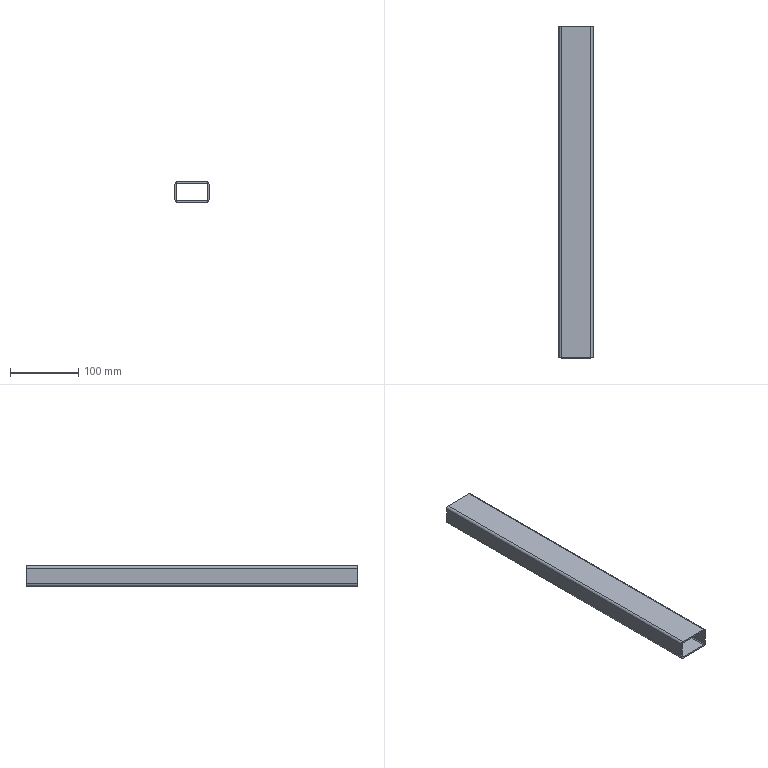Part | SolidWorks | features Extrusion 1 | 1 solid | 18 faces | box 50 x 488 x 30 mm | volume 164826 mm3 | plane 10 | cylinder 8 | commonest cylinder face diameters 2.3 x4 6.9 x4
STEP:
#1=CARTESIAN_POINT('',(25.,488.,-11.55));
#2=VERTEX_POINT('',#1);
#3=CARTESIAN_POINT('',(21.55,488.,-15.));
#4=VERTEX_POINT('',#3);
#5=CARTESIAN_POINT('',(21.55,488.,-11.55));
#6=DIRECTION('',(0.,1.,0.));
#7=DIRECTION('',(0.,0.,-1.));
#8=AXIS2_PLACEMENT_3D('',#5,#6,#7);
#9=CIRCLE('',#8,3.45);
#10=EDGE_CURVE('',#2,#4,#9,.T.);
#11=ORIENTED_EDGE('',*,*,#10,.T.);
#12=CARTESIAN_POINT('',(-21.55,488.,-15.));
#13=VERTEX_POINT('',#12);
#14=CARTESIAN_POINT('',(-21.55,488.,-15.));
#15=DIRECTION('',(-1.,0.,0.));
#16=VECTOR('',#15,1000.);
#17=LINE('',#14,#16);
#18=EDGE_CURVE('',#4,#13,#17,.T.);
#19=ORIENTED_EDGE('',*,*,#18,.T.);
#20=CARTESIAN_POINT('',(-25.,488.,-11.55));
#21=VERTEX_POINT('',#20);
#22=CARTESIAN_POINT('',(-21.55,488.,-11.55));
#23=DIRECTION('',(0.,1.,0.));
#24=DIRECTION('',(0.,0.,-1.));
#25=AXIS2_PLACEMENT_3D('',#22,#23,#24);
#26=CIRCLE('',#25,3.45);
#27=EDGE_CURVE('',#13,#21,#26,.T.);
#28=ORIENTED_EDGE('',*,*,#27,.T.);
#29=CARTESIAN_POINT('',(-25.,488.,11.55));
#30=VERTEX_POINT('',#29);
#31=CARTESIAN_POINT('',(-25.,488.,11.55));
#32=DIRECTION('',(0.,0.,1.));
#33=VECTOR('',#32,1000.);
#34=LINE('',#31,#33);
#35=EDGE_CURVE('',#21,#30,#34,.T.);
#36=ORIENTED_EDGE('',*,*,#35,.T.);
#37=CARTESIAN_POINT('',(-21.55,488.,15.));
#38=VERTEX_POINT('',#37);
#39=CARTESIAN_POINT('',(-21.55,488.,11.55));
#40=DIRECTION('',(0.,1.,0.));
#41=DIRECTION('',(0.,0.,-1.));
#42=AXIS2_PLACEMENT_3D('',#39,#40,#41);
#43=CIRCLE('',#42,3.45);
#44=EDGE_CURVE('',#30,#38,#43,.T.);
#45=ORIENTED_EDGE('',*,*,#44,.T.);
#46=CARTESIAN_POINT('',(21.55,488.,15.));
#47=VERTEX_POINT('',#46);
#48=CARTESIAN_POINT('',(-21.55,488.,15.));
#49=DIRECTION('',(1.,0.,0.));
#50=VECTOR('',#49,1000.);
#51=LINE('',#48,#50);
#52=EDGE_CURVE('',#38,#47,#51,.T.);
#53=ORIENTED_EDGE('',*,*,#52,.T.);
#54=CARTESIAN_POINT('',(25.,488.,11.55));
#55=VERTEX_POINT('',#54);
#56=CARTESIAN_POINT('',(21.55,488.,11.55));
#57=DIRECTION('',(0.,1.,0.));
#58=DIRECTION('',(0.,0.,1.));
#59=AXIS2_PLACEMENT_3D('',#56,#57,#58);
#60=CIRCLE('',#59,3.45);
#61=EDGE_CURVE('',#47,#55,#60,.T.);
#62=ORIENTED_EDGE('',*,*,#61,.T.);
#63=CARTESIAN_POINT('',(25.,488.,11.55));
#64=DIRECTION('',(0.,0.,-1.));
#65=VECTOR('',#64,1000.);
#66=LINE('',#63,#65);
#67=EDGE_CURVE('',#55,#2,#66,.T.);
#68=ORIENTED_EDGE('',*,*,#67,.T.);
#69=EDGE_LOOP('',(#11,#19,#28,#36,#45,#53,#62,#68));
#70=FACE_OUTER_BOUND('',#69,.T.);
#71=CARTESIAN_POINT('',(-22.7,488.,11.55));
#72=VERTEX_POINT('',#71);
#73=CARTESIAN_POINT('',(-21.55,488.,12.7));
#74=VERTEX_POINT('',#73);
#75=CARTESIAN_POINT('',(-21.55,488.,11.55));
#76=DIRECTION('',(0.,1.,0.));
#77=DIRECTION('',(0.,0.,-1.));
#78=AXIS2_PLACEMENT_3D('',#75,#76,#77);
#79=CIRCLE('',#78,1.15);
#80=EDGE_CURVE('',#72,#74,#79,.T.);
#81=ORIENTED_EDGE('',*,*,#80,.F.);
#82=CARTESIAN_POINT('',(-22.7,488.,-11.55));
#83=VERTEX_POINT('',#82);
#84=CARTESIAN_POINT('',(-22.7,488.,11.55));
#85=DIRECTION('',(0.,0.,1.));
#86=VECTOR('',#85,1000.);
#87=LINE('',#84,#86);
#88=EDGE_CURVE('',#83,#72,#87,.T.);
#89=ORIENTED_EDGE('',*,*,#88,.F.);
#90=CARTESIAN_POINT('',(-21.55,488.,-12.7));
#91=VERTEX_POINT('',#90);
#92=CARTESIAN_POINT('',(-21.55,488.,-11.55));
#93=DIRECTION('',(0.,1.,0.));
#94=DIRECTION('',(0.,0.,-1.));
#95=AXIS2_PLACEMENT_3D('',#92,#93,#94);
#96=CIRCLE('',#95,1.15);
#97=EDGE_CURVE('',#91,#83,#96,.T.);
#98=ORIENTED_EDGE('',*,*,#97,.F.);
#99=CARTESIAN_POINT('',(21.55,488.,-12.7));
#100=VERTEX_POINT('',#99);
#101=CARTESIAN_POINT('',(-21.55,488.,-12.7));
#102=DIRECTION('',(-1.,0.,0.));
#103=VECTOR('',#102,1000.);
#104=LINE('',#101,#103);
#105=EDGE_CURVE('',#100,#91,#104,.T.);
#106=ORIENTED_EDGE('',*,*,#105,.F.);
#107=CARTESIAN_POINT('',(22.7,488.,-11.55));
#108=VERTEX_POINT('',#107);
#109=CARTESIAN_POINT('',(21.55,488.,-11.55));
#110=DIRECTION('',(0.,1.,0.));
#111=DIRECTION('',(0.,0.,-1.));
#112=AXIS2_PLACEMENT_3D('',#109,#110,#111);
#113=CIRCLE('',#112,1.15);
#114=EDGE_CURVE('',#108,#100,#113,.T.);
#115=ORIENTED_EDGE('',*,*,#114,.F.);
#116=CARTESIAN_POINT('',(22.7,488.,11.55));
#117=VERTEX_POINT('',#116);
#118=CARTESIAN_POINT('',(22.7,488.,11.55));
#119=DIRECTION('',(0.,0.,-1.));
#120=VECTOR('',#119,1000.);
#121=LINE('',#118,#120);
#122=EDGE_CURVE('',#117,#108,#121,.T.);
#123=ORIENTED_EDGE('',*,*,#122,.F.);
#124=CARTESIAN_POINT('',(21.55,488.,12.7));
#125=VERTEX_POINT('',#124);
#126=CARTESIAN_POINT('',(21.55,488.,11.55));
#127=DIRECTION('',(0.,1.,0.));
#128=DIRECTION('',(0.,0.,1.));
#129=AXIS2_PLACEMENT_3D('',#126,#127,#128);
#130=CIRCLE('',#129,1.15);
#131=EDGE_CURVE('',#125,#117,#130,.T.);
#132=ORIENTED_EDGE('',*,*,#131,.F.);
#133=CARTESIAN_POINT('',(-21.55,488.,12.7));
#134=DIRECTION('',(1.,0.,0.));
#135=VECTOR('',#134,1000.);
#136=LINE('',#133,#135);
#137=EDGE_CURVE('',#74,#125,#136,.T.);
#138=ORIENTED_EDGE('',*,*,#137,.F.);
#139=EDGE_LOOP('',(#81,#89,#98,#106,#115,#123,#132,#138));
#140=FACE_BOUND('',#139,.T.);
#141=CARTESIAN_POINT('',(21.55,488.,-11.55));
#142=DIRECTION('',(0.,-1.,0.));
#143=DIRECTION('',(0.,0.,-1.));
#144=AXIS2_PLACEMENT_3D('',#141,#142,#143);
#145=PLANE('',#144);
#146=ADVANCED_FACE('',(#70,#140),#145,.F.);
#147=CARTESIAN_POINT('',(25.,0.,-11.55));
#148=VERTEX_POINT('',#147);
#149=CARTESIAN_POINT('',(21.55,0.,-15.));
#150=VERTEX_POINT('',#149);
#151=CARTESIAN_POINT('',(21.55,0.,-11.55));
#152=DIRECTION('',(0.,1.,0.));
#153=DIRECTION('',(0.,0.,-1.));
#154=AXIS2_PLACEMENT_3D('',#151,#152,#153);
#155=CIRCLE('',#154,3.45);
#156=EDGE_CURVE('',#148,#150,#155,.T.);
#157=ORIENTED_EDGE('',*,*,#156,.F.);
#158=CARTESIAN_POINT('',(25.,0.,11.55));
#159=VERTEX_POINT('',#158);
#160=CARTESIAN_POINT('',(25.,0.,11.55));
#161=DIRECTION('',(0.,0.,-1.));
#162=VECTOR('',#161,1000.);
#163=LINE('',#160,#162);
#164=EDGE_CURVE('',#159,#148,#163,.T.);
#165=ORIENTED_EDGE('',*,*,#164,.F.);
#166=CARTESIAN_POINT('',(21.55,0.,15.));
#167=VERTEX_POINT('',#166);
#168=CARTESIAN_POINT('',(21.55,0.,11.55));
#169=DIRECTION('',(0.,1.,0.));
#170=DIRECTION('',(0.,0.,1.));
#171=AXIS2_PLACEMENT_3D('',#168,#169,#170);
#172=CIRCLE('',#171,3.45);
#173=EDGE_CURVE('',#167,#159,#172,.T.);
#174=ORIENTED_EDGE('',*,*,#173,.F.);
#175=CARTESIAN_POINT('',(-21.55,0.,15.));
#176=VERTEX_POINT('',#175);
#177=CARTESIAN_POINT('',(-21.55,0.,15.));
#178=DIRECTION('',(1.,0.,0.));
#179=VECTOR('',#178,1000.);
#180=LINE('',#177,#179);
#181=EDGE_CURVE('',#176,#167,#180,.T.);
#182=ORIENTED_EDGE('',*,*,#181,.F.);
#183=CARTESIAN_POINT('',(-25.,0.,11.55));
#184=VERTEX_POINT('',#183);
#185=CARTESIAN_POINT('',(-21.55,0.,11.55));
#186=DIRECTION('',(0.,1.,0.));
#187=DIRECTION('',(0.,0.,-1.));
#188=AXIS2_PLACEMENT_3D('',#185,#186,#187);
#189=CIRCLE('',#188,3.45);
#190=EDGE_CURVE('',#184,#176,#189,.T.);
#191=ORIENTED_EDGE('',*,*,#190,.F.);
#192=CARTESIAN_POINT('',(-25.,0.,-11.55));
#193=VERTEX_POINT('',#192);
#194=CARTESIAN_POINT('',(-25.,0.,11.55));
#195=DIRECTION('',(0.,0.,1.));
#196=VECTOR('',#195,1000.);
#197=LINE('',#194,#196);
#198=EDGE_CURVE('',#193,#184,#197,.T.);
#199=ORIENTED_EDGE('',*,*,#198,.F.);
#200=CARTESIAN_POINT('',(-21.55,0.,-15.));
#201=VERTEX_POINT('',#200);
#202=CARTESIAN_POINT('',(-21.55,0.,-11.55));
#203=DIRECTION('',(0.,1.,0.));
#204=DIRECTION('',(0.,0.,-1.));
#205=AXIS2_PLACEMENT_3D('',#202,#203,#204);
#206=CIRCLE('',#205,3.45);
#207=EDGE_CURVE('',#201,#193,#206,.T.);
#208=ORIENTED_EDGE('',*,*,#207,.F.);
#209=CARTESIAN_POINT('',(-21.55,0.,-15.));
#210=DIRECTION('',(-1.,0.,0.));
#211=VECTOR('',#210,1000.);
#212=LINE('',#209,#211);
#213=EDGE_CURVE('',#150,#201,#212,.T.);
#214=ORIENTED_EDGE('',*,*,#213,.F.);
#215=EDGE_LOOP('',(#157,#165,#174,#182,#191,#199,#208,#214));
#216=FACE_OUTER_BOUND('',#215,.T.);
#217=CARTESIAN_POINT('',(-22.7,0.,-11.55));
#218=VERTEX_POINT('',#217);
#219=CARTESIAN_POINT('',(-22.7,0.,11.55));
#220=VERTEX_POINT('',#219);
#221=CARTESIAN_POINT('',(-22.7,0.,11.55));
#222=DIRECTION('',(0.,0.,1.));
#223=VECTOR('',#222,1000.);
#224=LINE('',#221,#223);
#225=EDGE_CURVE('',#218,#220,#224,.T.);
#226=ORIENTED_EDGE('',*,*,#225,.T.);
#227=CARTESIAN_POINT('',(-21.55,0.,12.7));
#228=VERTEX_POINT('',#227);
#229=CARTESIAN_POINT('',(-21.55,0.,11.55));
#230=DIRECTION('',(0.,1.,0.));
#231=DIRECTION('',(0.,0.,-1.));
#232=AXIS2_PLACEMENT_3D('',#229,#230,#231);
#233=CIRCLE('',#232,1.15);
#234=EDGE_CURVE('',#220,#228,#233,.T.);
#235=ORIENTED_EDGE('',*,*,#234,.T.);
#236=CARTESIAN_POINT('',(21.55,0.,12.7));
#237=VERTEX_POINT('',#236);
#238=CARTESIAN_POINT('',(-21.55,0.,12.7));
#239=DIRECTION('',(1.,0.,0.));
#240=VECTOR('',#239,1000.);
#241=LINE('',#238,#240);
#242=EDGE_CURVE('',#228,#237,#241,.T.);
#243=ORIENTED_EDGE('',*,*,#242,.T.);
#244=CARTESIAN_POINT('',(22.7,0.,11.55));
#245=VERTEX_POINT('',#244);
#246=CARTESIAN_POINT('',(21.55,0.,11.55));
#247=DIRECTION('',(0.,1.,0.));
#248=DIRECTION('',(0.,0.,1.));
#249=AXIS2_PLACEMENT_3D('',#246,#247,#248);
#250=CIRCLE('',#249,1.15);
#251=EDGE_CURVE('',#237,#245,#250,.T.);
#252=ORIENTED_EDGE('',*,*,#251,.T.);
#253=CARTESIAN_POINT('',(22.7,0.,-11.55));
#254=VERTEX_POINT('',#253);
#255=CARTESIAN_POINT('',(22.7,0.,11.55));
#256=DIRECTION('',(0.,0.,-1.));
#257=VECTOR('',#256,1000.);
#258=LINE('',#255,#257);
#259=EDGE_CURVE('',#245,#254,#258,.T.);
#260=ORIENTED_EDGE('',*,*,#259,.T.);
#261=CARTESIAN_POINT('',(21.55,0.,-12.7));
#262=VERTEX_POINT('',#261);
#263=CARTESIAN_POINT('',(21.55,0.,-11.55));
#264=DIRECTION('',(0.,1.,0.));
#265=DIRECTION('',(0.,0.,-1.));
#266=AXIS2_PLACEMENT_3D('',#263,#264,#265);
#267=CIRCLE('',#266,1.15);
#268=EDGE_CURVE('',#254,#262,#267,.T.);
#269=ORIENTED_EDGE('',*,*,#268,.T.);
#270=CARTESIAN_POINT('',(-21.55,0.,-12.7));
#271=VERTEX_POINT('',#270);
#272=CARTESIAN_POINT('',(-21.55,0.,-12.7));
#273=DIRECTION('',(-1.,0.,0.));
#274=VECTOR('',#273,1000.);
#275=LINE('',#272,#274);
#276=EDGE_CURVE('',#262,#271,#275,.T.);
#277=ORIENTED_EDGE('',*,*,#276,.T.);
#278=CARTESIAN_POINT('',(-21.55,0.,-11.55));
#279=DIRECTION('',(0.,1.,0.));
#280=DIRECTION('',(0.,0.,-1.));
#281=AXIS2_PLACEMENT_3D('',#278,#279,#280);
#282=CIRCLE('',#281,1.15);
#283=EDGE_CURVE('',#271,#218,#282,.T.);
#284=ORIENTED_EDGE('',*,*,#283,.T.);
#285=EDGE_LOOP('',(#226,#235,#243,#252,#260,#269,#277,#284));
#286=FACE_BOUND('',#285,.T.);
#287=CARTESIAN_POINT('',(21.55,0.,-11.55));
#288=DIRECTION('',(0.,-1.,0.));
#289=DIRECTION('',(0.,0.,-1.));
#290=AXIS2_PLACEMENT_3D('',#287,#288,#289);
#291=PLANE('',#290);
#292=ADVANCED_FACE('',(#216,#286),#291,.T.);
#293=ORIENTED_EDGE('',*,*,#156,.T.);
#294=CARTESIAN_POINT('',(21.55,488.,-15.));
#295=DIRECTION('',(0.,-1.,0.));
#296=VECTOR('',#295,1000.);
#297=LINE('',#294,#296);
#298=EDGE_CURVE('',#4,#150,#297,.T.);
#299=ORIENTED_EDGE('',*,*,#298,.F.);
#300=ORIENTED_EDGE('',*,*,#10,.F.);
#301=CARTESIAN_POINT('',(25.,488.,-11.55));
#302=DIRECTION('',(0.,-1.,0.));
#303=VECTOR('',#302,1000.);
#304=LINE('',#301,#303);
#305=EDGE_CURVE('',#2,#148,#304,.T.);
#306=ORIENTED_EDGE('',*,*,#305,.T.);
#307=EDGE_LOOP('',(#293,#299,#300,#306));
#308=FACE_OUTER_BOUND('',#307,.T.);
#309=CARTESIAN_POINT('',(21.55,488.,-11.55));
#310=DIRECTION('',(0.,-1.,0.));
#311=DIRECTION('',(0.,0.,-1.));
#312=AXIS2_PLACEMENT_3D('',#309,#310,#311);
#313=CYLINDRICAL_SURFACE('',#312,3.45);
#314=ADVANCED_FACE('',(#308),#313,.T.);
#315=ORIENTED_EDGE('',*,*,#213,.T.);
#316=CARTESIAN_POINT('',(-21.55,488.,-15.));
#317=DIRECTION('',(0.,-1.,0.));
#318=VECTOR('',#317,1000.);
#319=LINE('',#316,#318);
#320=EDGE_CURVE('',#13,#201,#319,.T.);
#321=ORIENTED_EDGE('',*,*,#320,.F.);
#322=ORIENTED_EDGE('',*,*,#18,.F.);
#323=ORIENTED_EDGE('',*,*,#298,.T.);
#324=EDGE_LOOP('',(#315,#321,#322,#323));
#325=FACE_OUTER_BOUND('',#324,.T.);
#326=CARTESIAN_POINT('',(-21.55,488.,-15.));
#327=DIRECTION('',(0.,0.,1.));
#328=DIRECTION('',(1.,0.,0.));
#329=AXIS2_PLACEMENT_3D('',#326,#327,#328);
#330=PLANE('',#329);
#331=ADVANCED_FACE('',(#325),#330,.F.);
#332=ORIENTED_EDGE('',*,*,#207,.T.);
#333=CARTESIAN_POINT('',(-25.,488.,-11.55));
#334=DIRECTION('',(0.,-1.,0.));
#335=VECTOR('',#334,1000.);
#336=LINE('',#333,#335);
#337=EDGE_CURVE('',#21,#193,#336,.T.);
#338=ORIENTED_EDGE('',*,*,#337,.F.);
#339=ORIENTED_EDGE('',*,*,#27,.F.);
#340=ORIENTED_EDGE('',*,*,#320,.T.);
#341=EDGE_LOOP('',(#332,#338,#339,#340));
#342=FACE_OUTER_BOUND('',#341,.T.);
#343=CARTESIAN_POINT('',(-21.55,488.,-11.55));
#344=DIRECTION('',(0.,-1.,0.));
#345=DIRECTION('',(0.,0.,-1.));
#346=AXIS2_PLACEMENT_3D('',#343,#344,#345);
#347=CYLINDRICAL_SURFACE('',#346,3.45);
#348=ADVANCED_FACE('',(#342),#347,.T.);
#349=ORIENTED_EDGE('',*,*,#198,.T.);
#350=CARTESIAN_POINT('',(-25.,488.,11.55));
#351=DIRECTION('',(0.,-1.,0.));
#352=VECTOR('',#351,1000.);
#353=LINE('',#350,#352);
#354=EDGE_CURVE('',#30,#184,#353,.T.);
#355=ORIENTED_EDGE('',*,*,#354,.F.);
#356=ORIENTED_EDGE('',*,*,#35,.F.);
#357=ORIENTED_EDGE('',*,*,#337,.T.);
#358=EDGE_LOOP('',(#349,#355,#356,#357));
#359=FACE_OUTER_BOUND('',#358,.T.);
#360=CARTESIAN_POINT('',(-25.,488.,11.55));
#361=DIRECTION('',(1.,0.,0.));
#362=DIRECTION('',(0.,0.,-1.));
#363=AXIS2_PLACEMENT_3D('',#360,#361,#362);
#364=PLANE('',#363);
#365=ADVANCED_FACE('',(#359),#364,.F.);
#366=ORIENTED_EDGE('',*,*,#190,.T.);
#367=CARTESIAN_POINT('',(-21.55,488.,15.));
#368=DIRECTION('',(0.,-1.,0.));
#369=VECTOR('',#368,1000.);
#370=LINE('',#367,#369);
#371=EDGE_CURVE('',#38,#176,#370,.T.);
#372=ORIENTED_EDGE('',*,*,#371,.F.);
#373=ORIENTED_EDGE('',*,*,#44,.F.);
#374=ORIENTED_EDGE('',*,*,#354,.T.);
#375=EDGE_LOOP('',(#366,#372,#373,#374));
#376=FACE_OUTER_BOUND('',#375,.T.);
#377=CARTESIAN_POINT('',(-21.55,488.,11.55));
#378=DIRECTION('',(0.,-1.,0.));
#379=DIRECTION('',(0.,0.,-1.));
#380=AXIS2_PLACEMENT_3D('',#377,#378,#379);
#381=CYLINDRICAL_SURFACE('',#380,3.45);
#382=ADVANCED_FACE('',(#376),#381,.T.);
#383=ORIENTED_EDGE('',*,*,#181,.T.);
#384=CARTESIAN_POINT('',(21.55,488.,15.));
#385=DIRECTION('',(0.,-1.,0.));
#386=VECTOR('',#385,1000.);
#387=LINE('',#384,#386);
#388=EDGE_CURVE('',#47,#167,#387,.T.);
#389=ORIENTED_EDGE('',*,*,#388,.F.);
#390=ORIENTED_EDGE('',*,*,#52,.F.);
#391=ORIENTED_EDGE('',*,*,#371,.T.);
#392=EDGE_LOOP('',(#383,#389,#390,#391));
#393=FACE_OUTER_BOUND('',#392,.T.);
#394=CARTESIAN_POINT('',(-21.55,488.,15.));
#395=DIRECTION('',(0.,0.,-1.));
#396=DIRECTION('',(-1.,0.,0.));
#397=AXIS2_PLACEMENT_3D('',#394,#395,#396);
#398=PLANE('',#397);
#399=ADVANCED_FACE('',(#393),#398,.F.);
#400=ORIENTED_EDGE('',*,*,#173,.T.);
#401=CARTESIAN_POINT('',(25.,488.,11.55));
#402=DIRECTION('',(0.,-1.,0.));
#403=VECTOR('',#402,1000.);
#404=LINE('',#401,#403);
#405=EDGE_CURVE('',#55,#159,#404,.T.);
#406=ORIENTED_EDGE('',*,*,#405,.F.);
#407=ORIENTED_EDGE('',*,*,#61,.F.);
#408=ORIENTED_EDGE('',*,*,#388,.T.);
#409=EDGE_LOOP('',(#400,#406,#407,#408));
#410=FACE_OUTER_BOUND('',#409,.T.);
#411=CARTESIAN_POINT('',(21.55,488.,11.55));
#412=DIRECTION('',(0.,-1.,0.));
#413=DIRECTION('',(0.,0.,-1.));
#414=AXIS2_PLACEMENT_3D('',#411,#412,#413);
#415=CYLINDRICAL_SURFACE('',#414,3.45);
#416=ADVANCED_FACE('',(#410),#415,.T.);
#417=ORIENTED_EDGE('',*,*,#164,.T.);
#418=ORIENTED_EDGE('',*,*,#305,.F.);
#419=ORIENTED_EDGE('',*,*,#67,.F.);
#420=ORIENTED_EDGE('',*,*,#405,.T.);
#421=EDGE_LOOP('',(#417,#418,#419,#420));
#422=FACE_OUTER_BOUND('',#421,.T.);
#423=CARTESIAN_POINT('',(25.,488.,11.55));
#424=DIRECTION('',(-1.,0.,0.));
#425=DIRECTION('',(0.,0.,1.));
#426=AXIS2_PLACEMENT_3D('',#423,#424,#425);
#427=PLANE('',#426);
#428=ADVANCED_FACE('',(#422),#427,.F.);
#429=ORIENTED_EDGE('',*,*,#234,.F.);
#430=CARTESIAN_POINT('',(-22.7,488.,11.55));
#431=DIRECTION('',(0.,-1.,0.));
#432=VECTOR('',#431,1000.);
#433=LINE('',#430,#432);
#434=EDGE_CURVE('',#72,#220,#433,.T.);
#435=ORIENTED_EDGE('',*,*,#434,.F.);
#436=ORIENTED_EDGE('',*,*,#80,.T.);
#437=CARTESIAN_POINT('',(-21.55,488.,12.7));
#438=DIRECTION('',(0.,-1.,0.));
#439=VECTOR('',#438,1000.);
#440=LINE('',#437,#439);
#441=EDGE_CURVE('',#74,#228,#440,.T.);
#442=ORIENTED_EDGE('',*,*,#441,.T.);
#443=EDGE_LOOP('',(#429,#435,#436,#442));
#444=FACE_OUTER_BOUND('',#443,.T.);
#445=CARTESIAN_POINT('',(-21.55,488.,11.55));
#446=DIRECTION('',(0.,-1.,0.));
#447=DIRECTION('',(0.,0.,-1.));
#448=AXIS2_PLACEMENT_3D('',#445,#446,#447);
#449=CYLINDRICAL_SURFACE('',#448,1.15);
#450=ADVANCED_FACE('',(#444),#449,.F.);
#451=ORIENTED_EDGE('',*,*,#242,.F.);
#452=ORIENTED_EDGE('',*,*,#441,.F.);
#453=ORIENTED_EDGE('',*,*,#137,.T.);
#454=CARTESIAN_POINT('',(21.55,488.,12.7));
#455=DIRECTION('',(0.,-1.,0.));
#456=VECTOR('',#455,1000.);
#457=LINE('',#454,#456);
#458=EDGE_CURVE('',#125,#237,#457,.T.);
#459=ORIENTED_EDGE('',*,*,#458,.T.);
#460=EDGE_LOOP('',(#451,#452,#453,#459));
#461=FACE_OUTER_BOUND('',#460,.T.);
#462=CARTESIAN_POINT('',(-21.55,488.,12.7));
#463=DIRECTION('',(0.,0.,-1.));
#464=DIRECTION('',(-1.,0.,0.));
#465=AXIS2_PLACEMENT_3D('',#462,#463,#464);
#466=PLANE('',#465);
#467=ADVANCED_FACE('',(#461),#466,.T.);
#468=ORIENTED_EDGE('',*,*,#251,.F.);
#469=ORIENTED_EDGE('',*,*,#458,.F.);
#470=ORIENTED_EDGE('',*,*,#131,.T.);
#471=CARTESIAN_POINT('',(22.7,488.,11.55));
#472=DIRECTION('',(0.,-1.,0.));
#473=VECTOR('',#472,1000.);
#474=LINE('',#471,#473);
#475=EDGE_CURVE('',#117,#245,#474,.T.);
#476=ORIENTED_EDGE('',*,*,#475,.T.);
#477=EDGE_LOOP('',(#468,#469,#470,#476));
#478=FACE_OUTER_BOUND('',#477,.T.);
#479=CARTESIAN_POINT('',(21.55,488.,11.55));
#480=DIRECTION('',(0.,-1.,0.));
#481=DIRECTION('',(0.,0.,-1.));
#482=AXIS2_PLACEMENT_3D('',#479,#480,#481);
#483=CYLINDRICAL_SURFACE('',#482,1.15);
#484=ADVANCED_FACE('',(#478),#483,.F.);
#485=ORIENTED_EDGE('',*,*,#259,.F.);
#486=ORIENTED_EDGE('',*,*,#475,.F.);
#487=ORIENTED_EDGE('',*,*,#122,.T.);
#488=CARTESIAN_POINT('',(22.7,488.,-11.55));
#489=DIRECTION('',(0.,-1.,0.));
#490=VECTOR('',#489,1000.);
#491=LINE('',#488,#490);
#492=EDGE_CURVE('',#108,#254,#491,.T.);
#493=ORIENTED_EDGE('',*,*,#492,.T.);
#494=EDGE_LOOP('',(#485,#486,#487,#493));
#495=FACE_OUTER_BOUND('',#494,.T.);
#496=CARTESIAN_POINT('',(22.7,488.,11.55));
#497=DIRECTION('',(-1.,0.,0.));
#498=DIRECTION('',(0.,0.,1.));
#499=AXIS2_PLACEMENT_3D('',#496,#497,#498);
#500=PLANE('',#499);
#501=ADVANCED_FACE('',(#495),#500,.T.);
#502=ORIENTED_EDGE('',*,*,#268,.F.);
#503=ORIENTED_EDGE('',*,*,#492,.F.);
#504=ORIENTED_EDGE('',*,*,#114,.T.);
#505=CARTESIAN_POINT('',(21.55,488.,-12.7));
#506=DIRECTION('',(0.,-1.,0.));
#507=VECTOR('',#506,1000.);
#508=LINE('',#505,#507);
#509=EDGE_CURVE('',#100,#262,#508,.T.);
#510=ORIENTED_EDGE('',*,*,#509,.T.);
#511=EDGE_LOOP('',(#502,#503,#504,#510));
#512=FACE_OUTER_BOUND('',#511,.T.);
#513=CARTESIAN_POINT('',(21.55,488.,-11.55));
#514=DIRECTION('',(0.,-1.,0.));
#515=DIRECTION('',(0.,0.,-1.));
#516=AXIS2_PLACEMENT_3D('',#513,#514,#515);
#517=CYLINDRICAL_SURFACE('',#516,1.15);
#518=ADVANCED_FACE('',(#512),#517,.F.);
#519=ORIENTED_EDGE('',*,*,#276,.F.);
#520=ORIENTED_EDGE('',*,*,#509,.F.);
#521=ORIENTED_EDGE('',*,*,#105,.T.);
#522=CARTESIAN_POINT('',(-21.55,488.,-12.7));
#523=DIRECTION('',(0.,-1.,0.));
#524=VECTOR('',#523,1000.);
#525=LINE('',#522,#524);
#526=EDGE_CURVE('',#91,#271,#525,.T.);
#527=ORIENTED_EDGE('',*,*,#526,.T.);
#528=EDGE_LOOP('',(#519,#520,#521,#527));
#529=FACE_OUTER_BOUND('',#528,.T.);
#530=CARTESIAN_POINT('',(-21.55,488.,-12.7));
#531=DIRECTION('',(0.,0.,1.));
#532=DIRECTION('',(1.,0.,0.));
#533=AXIS2_PLACEMENT_3D('',#530,#531,#532);
#534=PLANE('',#533);
#535=ADVANCED_FACE('',(#529),#534,.T.);
#536=ORIENTED_EDGE('',*,*,#283,.F.);
#537=ORIENTED_EDGE('',*,*,#526,.F.);
#538=ORIENTED_EDGE('',*,*,#97,.T.);
#539=CARTESIAN_POINT('',(-22.7,488.,-11.55));
#540=DIRECTION('',(0.,-1.,0.));
#541=VECTOR('',#540,1000.);
#542=LINE('',#539,#541);
#543=EDGE_CURVE('',#83,#218,#542,.T.);
#544=ORIENTED_EDGE('',*,*,#543,.T.);
#545=EDGE_LOOP('',(#536,#537,#538,#544));
#546=FACE_OUTER_BOUND('',#545,.T.);
#547=CARTESIAN_POINT('',(-21.55,488.,-11.55));
#548=DIRECTION('',(0.,-1.,0.));
#549=DIRECTION('',(0.,0.,-1.));
#550=AXIS2_PLACEMENT_3D('',#547,#548,#549);
#551=CYLINDRICAL_SURFACE('',#550,1.15);
#552=ADVANCED_FACE('',(#546),#551,.F.);
#553=ORIENTED_EDGE('',*,*,#225,.F.);
#554=ORIENTED_EDGE('',*,*,#543,.F.);
#555=ORIENTED_EDGE('',*,*,#88,.T.);
#556=ORIENTED_EDGE('',*,*,#434,.T.);
#557=EDGE_LOOP('',(#553,#554,#555,#556));
#558=FACE_OUTER_BOUND('',#557,.T.);
#559=CARTESIAN_POINT('',(-22.7,488.,11.55));
#560=DIRECTION('',(1.,0.,0.));
#561=DIRECTION('',(0.,0.,-1.));
#562=AXIS2_PLACEMENT_3D('',#559,#560,#561);
#563=PLANE('',#562);
#564=ADVANCED_FACE('',(#558),#563,.T.);
#565=CLOSED_SHELL('',(#146,#292,#314,#331,#348,#365,#382,#399,#416,#428,#450,#467,#484,#501,#518,#535,#552,#564));
#566=MANIFOLD_SOLID_BREP('',#565);
#567=CARTESIAN_POINT('',(0.,0.,0.));
#568=DIRECTION('',(0.,0.,1.));
#569=DIRECTION('',(1.,0.,0.));
#570=AXIS2_PLACEMENT_3D('',#567,#568,#569);
#571=(LENGTH_UNIT()NAMED_UNIT(*)SI_UNIT(.MILLI.,.METRE.));
#572=UNCERTAINTY_MEASURE_WITH_UNIT(LENGTH_MEASURE(0.00001),#571,'','');
#573=(NAMED_UNIT(*)PLANE_ANGLE_UNIT()SI_UNIT($,.RADIAN.));
#574=(NAMED_UNIT(*)SI_UNIT($,.STERADIAN.)SOLID_ANGLE_UNIT());
#575=(GEOMETRIC_REPRESENTATION_CONTEXT(3)GLOBAL_UNCERTAINTY_ASSIGNED_CONTEXT((#572))GLOBAL_UNIT_ASSIGNED_CONTEXT((#571,#573,#574))REPRESENTATION_CONTEXT('',''));
#576=ADVANCED_BREP_SHAPE_REPRESENTATION('',(#566,#570),#575);